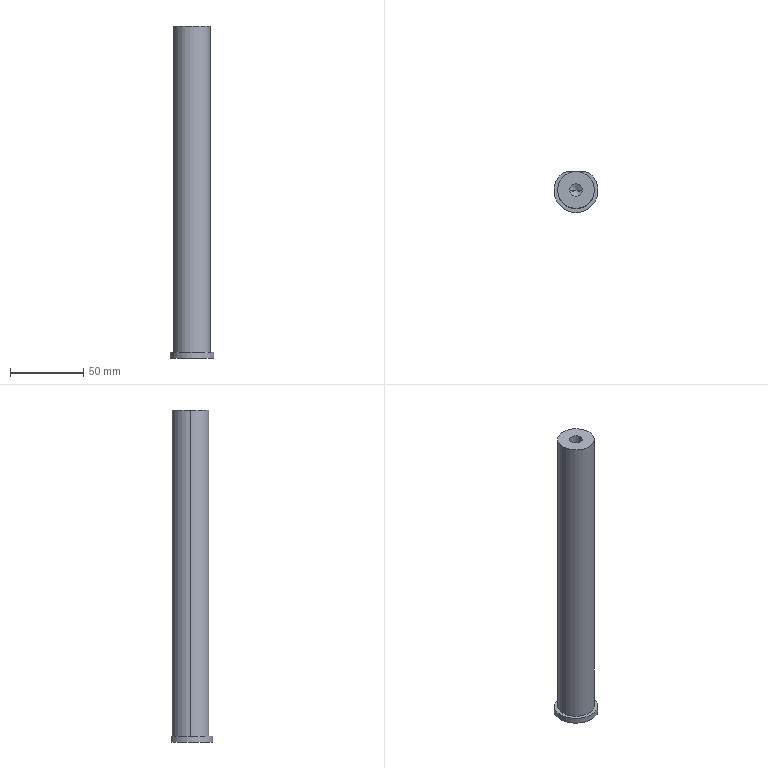Part | Creo | 1 solid | 13 faces | box 30 x 28 x 226 mm | volume 110529 mm3 | plane 6 | cylinder 5 | cone 2 | commonest cylinder face diameters 8.5 x2 25 x2 30 x1
STEP:
#1=CARTESIAN_POINT('',(0.,0.,0.));
#2=DIRECTION('',(0.,0.,1.));
#3=DIRECTION('',(1.,0.,0.));
#4=AXIS2_PLACEMENT_3D('',#1,#2,#3);
#5=CARTESIAN_POINT('',(108.255,195.804,-221.5));
#6=VERTEX_POINT('',#5);
#7=CARTESIAN_POINT('',(89.745,195.804,-221.5));
#8=VERTEX_POINT('',#7);
#9=CARTESIAN_POINT('',(99.,184.,-221.5));
#10=DIRECTION('',(0.,0.,-1.));
#11=DIRECTION('',(0.617,0.787,0.));
#12=AXIS2_PLACEMENT_3D('',#9,#10,#11);
#13=CIRCLE('',#12,15.);
#14=EDGE_CURVE('',#6,#8,#13,.T.);
#15=ORIENTED_EDGE('',*,*,#14,.F.);
#16=CARTESIAN_POINT('',(108.255,195.804,-225.5));
#17=VERTEX_POINT('',#16);
#18=CARTESIAN_POINT('',(108.255,195.804,-225.5));
#19=DIRECTION('',(0.,0.,1.));
#20=VECTOR('',#19,4.);
#21=LINE('',#18,#20);
#22=EDGE_CURVE('',#17,#6,#21,.T.);
#23=ORIENTED_EDGE('',*,*,#22,.F.);
#24=CARTESIAN_POINT('',(89.745,195.804,-225.5));
#25=VERTEX_POINT('',#24);
#26=CARTESIAN_POINT('',(99.,184.,-225.5));
#27=DIRECTION('',(0.,0.,1.));
#28=DIRECTION('',(-0.617,0.787,0.));
#29=AXIS2_PLACEMENT_3D('',#26,#27,#28);
#30=CIRCLE('',#29,15.);
#31=EDGE_CURVE('',#25,#17,#30,.T.);
#32=ORIENTED_EDGE('',*,*,#31,.F.);
#33=CARTESIAN_POINT('',(89.745,195.804,-221.5));
#34=DIRECTION('',(0.,0.,-1.));
#35=VECTOR('',#34,4.);
#36=LINE('',#33,#35);
#37=EDGE_CURVE('',#8,#25,#36,.T.);
#38=ORIENTED_EDGE('',*,*,#37,.F.);
#39=EDGE_LOOP('',(#15,#23,#32,#38));
#40=FACE_OUTER_BOUND('',#39,.F.);
#41=CARTESIAN_POINT('',(99.,184.,-221.5));
#42=DIRECTION('',(0.,0.,-1.));
#43=DIRECTION('',(1.,0.,0.));
#44=AXIS2_PLACEMENT_3D('',#41,#42,#43);
#45=CYLINDRICAL_SURFACE('',#44,15.);
#46=ADVANCED_FACE('',(#40),#45,.T.);
#47=CARTESIAN_POINT('',(104.792,197.,-221.5));
#48=VERTEX_POINT('',#47);
#49=CARTESIAN_POINT('',(93.208,197.,-221.5));
#50=VERTEX_POINT('',#49);
#51=CARTESIAN_POINT('',(104.792,197.,-221.5));
#52=DIRECTION('',(-1.,0.,0.));
#53=VECTOR('',#52,11.584);
#54=LINE('',#51,#53);
#55=EDGE_CURVE('',#48,#50,#54,.T.);
#56=ORIENTED_EDGE('',*,*,#55,.F.);
#57=CARTESIAN_POINT('',(108.255,195.804,-221.5));
#58=DIRECTION('',(-0.9452,0.3264,0.));
#59=VECTOR('',#58,3.664);
#60=LINE('',#57,#59);
#61=EDGE_CURVE('',#6,#48,#60,.T.);
#62=ORIENTED_EDGE('',*,*,#61,.F.);
#63=ORIENTED_EDGE('',*,*,#14,.T.);
#64=CARTESIAN_POINT('',(93.208,197.,-221.5));
#65=DIRECTION('',(-0.9452,-0.3264,0.));
#66=VECTOR('',#65,3.664);
#67=LINE('',#64,#66);
#68=EDGE_CURVE('',#50,#8,#67,.T.);
#69=ORIENTED_EDGE('',*,*,#68,.F.);
#70=EDGE_LOOP('',(#56,#62,#63,#69));
#71=FACE_OUTER_BOUND('',#70,.F.);
#72=CARTESIAN_POINT('',(111.5,184.,-221.5));
#73=VERTEX_POINT('',#72);
#74=CARTESIAN_POINT('',(86.5,184.,-221.5));
#75=VERTEX_POINT('',#74);
#76=CARTESIAN_POINT('',(99.,184.,-221.5));
#77=DIRECTION('',(0.,0.,-1.));
#78=DIRECTION('',(1.,0.,0.));
#79=AXIS2_PLACEMENT_3D('',#76,#77,#78);
#80=CIRCLE('',#79,12.5);
#81=EDGE_CURVE('',#73,#75,#80,.T.);
#82=ORIENTED_EDGE('',*,*,#81,.F.);
#83=CARTESIAN_POINT('',(99.,184.,-221.5));
#84=DIRECTION('',(0.,0.,-1.));
#85=DIRECTION('',(-1.,0.,0.));
#86=AXIS2_PLACEMENT_3D('',#83,#84,#85);
#87=CIRCLE('',#86,12.5);
#88=EDGE_CURVE('',#75,#73,#87,.T.);
#89=ORIENTED_EDGE('',*,*,#88,.F.);
#90=EDGE_LOOP('',(#82,#89));
#91=FACE_BOUND('',#90,.F.);
#92=CARTESIAN_POINT('',(99.,184.,-221.5));
#93=DIRECTION('',(0.,0.,1.));
#94=DIRECTION('',(-1.,0.,0.));
#95=AXIS2_PLACEMENT_3D('',#92,#93,#94);
#96=PLANE('',#95);
#97=ADVANCED_FACE('',(#71,#91),#96,.T.);
#98=CARTESIAN_POINT('',(86.5,184.,0.5));
#99=VERTEX_POINT('',#98);
#100=CARTESIAN_POINT('',(111.5,184.,0.5));
#101=VERTEX_POINT('',#100);
#102=CARTESIAN_POINT('',(99.,184.,0.5));
#103=DIRECTION('',(0.,0.,1.));
#104=DIRECTION('',(-1.,0.,0.));
#105=AXIS2_PLACEMENT_3D('',#102,#103,#104);
#106=CIRCLE('',#105,12.5);
#107=EDGE_CURVE('',#99,#101,#106,.T.);
#108=ORIENTED_EDGE('',*,*,#107,.T.);
#109=CARTESIAN_POINT('',(111.5,184.,-221.5));
#110=DIRECTION('',(0.,0.,1.));
#111=VECTOR('',#110,222.);
#112=LINE('',#109,#111);
#113=EDGE_CURVE('',#73,#101,#112,.T.);
#114=ORIENTED_EDGE('',*,*,#113,.F.);
#115=ORIENTED_EDGE('',*,*,#81,.T.);
#116=CARTESIAN_POINT('',(86.5,184.,-221.5));
#117=DIRECTION('',(0.,0.,1.));
#118=VECTOR('',#117,222.);
#119=LINE('',#116,#118);
#120=EDGE_CURVE('',#75,#99,#119,.T.);
#121=ORIENTED_EDGE('',*,*,#120,.T.);
#122=EDGE_LOOP('',(#108,#114,#115,#121));
#123=FACE_OUTER_BOUND('',#122,.F.);
#124=CARTESIAN_POINT('',(99.,184.,-221.5));
#125=DIRECTION('',(0.,0.,1.));
#126=DIRECTION('',(-1.,0.,0.));
#127=AXIS2_PLACEMENT_3D('',#124,#125,#126);
#128=CYLINDRICAL_SURFACE('',#127,12.5);
#129=ADVANCED_FACE('',(#123),#128,.T.);
#130=CARTESIAN_POINT('',(99.,184.,0.5));
#131=DIRECTION('',(0.,0.,1.));
#132=DIRECTION('',(1.,0.,0.));
#133=AXIS2_PLACEMENT_3D('',#130,#131,#132);
#134=CIRCLE('',#133,12.5);
#135=EDGE_CURVE('',#101,#99,#134,.T.);
#136=ORIENTED_EDGE('',*,*,#135,.F.);
#137=ORIENTED_EDGE('',*,*,#107,.F.);
#138=EDGE_LOOP('',(#136,#137));
#139=FACE_OUTER_BOUND('',#138,.F.);
#140=CARTESIAN_POINT('',(94.75,184.,0.5));
#141=VERTEX_POINT('',#140);
#142=CARTESIAN_POINT('',(103.25,184.,0.5));
#143=VERTEX_POINT('',#142);
#144=CARTESIAN_POINT('',(99.,184.,0.5));
#145=DIRECTION('',(0.,0.,-1.));
#146=DIRECTION('',(-1.,0.,0.));
#147=AXIS2_PLACEMENT_3D('',#144,#145,#146);
#148=CIRCLE('',#147,4.25);
#149=EDGE_CURVE('',#141,#143,#148,.T.);
#150=ORIENTED_EDGE('',*,*,#149,.F.);
#151=CARTESIAN_POINT('',(99.,184.,0.5));
#152=DIRECTION('',(0.,0.,-1.));
#153=DIRECTION('',(1.,0.,0.));
#154=AXIS2_PLACEMENT_3D('',#151,#152,#153);
#155=CIRCLE('',#154,4.25);
#156=EDGE_CURVE('',#143,#141,#155,.T.);
#157=ORIENTED_EDGE('',*,*,#156,.F.);
#158=EDGE_LOOP('',(#150,#157));
#159=FACE_BOUND('',#158,.F.);
#160=CARTESIAN_POINT('',(99.,184.,0.5));
#161=DIRECTION('',(0.,0.,1.));
#162=DIRECTION('',(-1.,0.,0.));
#163=AXIS2_PLACEMENT_3D('',#160,#161,#162);
#164=PLANE('',#163);
#165=ADVANCED_FACE('',(#139,#159),#164,.T.);
#166=CARTESIAN_POINT('',(103.25,184.,-19.5));
#167=VERTEX_POINT('',#166);
#168=CARTESIAN_POINT('',(94.75,184.,-19.5));
#169=VERTEX_POINT('',#168);
#170=CARTESIAN_POINT('',(99.,184.,-19.5));
#171=DIRECTION('',(0.,0.,1.));
#172=DIRECTION('',(1.,0.,0.));
#173=AXIS2_PLACEMENT_3D('',#170,#171,#172);
#174=CIRCLE('',#173,4.25);
#175=EDGE_CURVE('',#167,#169,#174,.T.);
#176=ORIENTED_EDGE('',*,*,#175,.T.);
#177=CARTESIAN_POINT('',(94.75,184.,0.5));
#178=DIRECTION('',(0.,0.,-1.));
#179=VECTOR('',#178,20.);
#180=LINE('',#177,#179);
#181=EDGE_CURVE('',#141,#169,#180,.T.);
#182=ORIENTED_EDGE('',*,*,#181,.F.);
#183=ORIENTED_EDGE('',*,*,#149,.T.);
#184=CARTESIAN_POINT('',(103.25,184.,0.5));
#185=DIRECTION('',(0.,0.,-1.));
#186=VECTOR('',#185,20.);
#187=LINE('',#184,#186);
#188=EDGE_CURVE('',#143,#167,#187,.T.);
#189=ORIENTED_EDGE('',*,*,#188,.T.);
#190=EDGE_LOOP('',(#176,#182,#183,#189));
#191=FACE_OUTER_BOUND('',#190,.F.);
#192=CARTESIAN_POINT('',(99.,184.,0.5));
#193=DIRECTION('',(0.,0.,-1.));
#194=DIRECTION('',(-1.,0.,0.));
#195=AXIS2_PLACEMENT_3D('',#192,#193,#194);
#196=CYLINDRICAL_SURFACE('',#195,4.25);
#197=ADVANCED_FACE('',(#191),#196,.F.);
#198=ORIENTED_EDGE('',*,*,#175,.F.);
#199=CARTESIAN_POINT('',(99.,184.,-22.054));
#200=VERTEX_POINT('',#199);
#201=CARTESIAN_POINT('',(99.,184.,-22.054));
#202=DIRECTION('',(0.8572,0.,0.515));
#203=VECTOR('',#202,4.958);
#204=LINE('',#201,#203);
#205=EDGE_CURVE('',#200,#167,#204,.T.);
#206=ORIENTED_EDGE('',*,*,#205,.F.);
#207=CARTESIAN_POINT('',(99.,184.,-22.054));
#208=DIRECTION('',(-0.8572,0.,0.515));
#209=VECTOR('',#208,4.958);
#210=LINE('',#207,#209);
#211=EDGE_CURVE('',#200,#169,#210,.T.);
#212=ORIENTED_EDGE('',*,*,#211,.T.);
#213=EDGE_LOOP('',(#198,#206,#212));
#214=FACE_OUTER_BOUND('',#213,.F.);
#215=CARTESIAN_POINT('',(99.,184.,-20.706));
#216=DIRECTION('',(0.,0.,1.));
#217=DIRECTION('',(1.,0.,0.));
#218=AXIS2_PLACEMENT_3D('',#215,#216,#217);
#219=CONICAL_SURFACE('',#218,2.243,59.);
#220=ADVANCED_FACE('',(#214),#219,.F.);
#221=CARTESIAN_POINT('',(99.,184.,-19.5));
#222=DIRECTION('',(0.,0.,1.));
#223=DIRECTION('',(-1.,0.,0.));
#224=AXIS2_PLACEMENT_3D('',#221,#222,#223);
#225=CIRCLE('',#224,4.25);
#226=EDGE_CURVE('',#169,#167,#225,.T.);
#227=ORIENTED_EDGE('',*,*,#226,.F.);
#228=ORIENTED_EDGE('',*,*,#211,.F.);
#229=ORIENTED_EDGE('',*,*,#205,.T.);
#230=EDGE_LOOP('',(#227,#228,#229));
#231=FACE_OUTER_BOUND('',#230,.F.);
#232=CARTESIAN_POINT('',(99.,184.,-20.706));
#233=DIRECTION('',(0.,0.,1.));
#234=DIRECTION('',(1.,0.,0.));
#235=AXIS2_PLACEMENT_3D('',#232,#233,#234);
#236=CONICAL_SURFACE('',#235,2.243,59.);
#237=ADVANCED_FACE('',(#231),#236,.F.);
#238=ORIENTED_EDGE('',*,*,#226,.T.);
#239=ORIENTED_EDGE('',*,*,#188,.F.);
#240=ORIENTED_EDGE('',*,*,#156,.T.);
#241=ORIENTED_EDGE('',*,*,#181,.T.);
#242=EDGE_LOOP('',(#238,#239,#240,#241));
#243=FACE_OUTER_BOUND('',#242,.F.);
#244=CARTESIAN_POINT('',(99.,184.,0.5));
#245=DIRECTION('',(0.,0.,-1.));
#246=DIRECTION('',(-1.,0.,0.));
#247=AXIS2_PLACEMENT_3D('',#244,#245,#246);
#248=CYLINDRICAL_SURFACE('',#247,4.25);
#249=ADVANCED_FACE('',(#243),#248,.F.);
#250=ORIENTED_EDGE('',*,*,#135,.T.);
#251=ORIENTED_EDGE('',*,*,#120,.F.);
#252=ORIENTED_EDGE('',*,*,#88,.T.);
#253=ORIENTED_EDGE('',*,*,#113,.T.);
#254=EDGE_LOOP('',(#250,#251,#252,#253));
#255=FACE_OUTER_BOUND('',#254,.F.);
#256=CARTESIAN_POINT('',(99.,184.,-221.5));
#257=DIRECTION('',(0.,0.,1.));
#258=DIRECTION('',(-1.,0.,0.));
#259=AXIS2_PLACEMENT_3D('',#256,#257,#258);
#260=CYLINDRICAL_SURFACE('',#259,12.5);
#261=ADVANCED_FACE('',(#255),#260,.T.);
#262=CARTESIAN_POINT('',(104.792,197.,-225.5));
#263=VERTEX_POINT('',#262);
#264=CARTESIAN_POINT('',(93.208,197.,-225.5));
#265=VERTEX_POINT('',#264);
#266=CARTESIAN_POINT('',(104.792,197.,-225.5));
#267=DIRECTION('',(-1.,0.,0.));
#268=VECTOR('',#267,11.584);
#269=LINE('',#266,#268);
#270=EDGE_CURVE('',#263,#265,#269,.T.);
#271=ORIENTED_EDGE('',*,*,#270,.F.);
#272=CARTESIAN_POINT('',(104.792,197.,-225.5));
#273=DIRECTION('',(0.,0.,1.));
#274=VECTOR('',#273,4.);
#275=LINE('',#272,#274);
#276=EDGE_CURVE('',#263,#48,#275,.T.);
#277=ORIENTED_EDGE('',*,*,#276,.T.);
#278=ORIENTED_EDGE('',*,*,#55,.T.);
#279=CARTESIAN_POINT('',(93.208,197.,-221.5));
#280=DIRECTION('',(0.,0.,-1.));
#281=VECTOR('',#280,4.);
#282=LINE('',#279,#281);
#283=EDGE_CURVE('',#50,#265,#282,.T.);
#284=ORIENTED_EDGE('',*,*,#283,.T.);
#285=EDGE_LOOP('',(#271,#277,#278,#284));
#286=FACE_OUTER_BOUND('',#285,.F.);
#287=CARTESIAN_POINT('',(99.,197.,-225.5));
#288=DIRECTION('',(0.,1.,0.));
#289=DIRECTION('',(0.,0.,1.));
#290=AXIS2_PLACEMENT_3D('',#287,#288,#289);
#291=PLANE('',#290);
#292=ADVANCED_FACE('',(#286),#291,.T.);
#293=ORIENTED_EDGE('',*,*,#31,.T.);
#294=CARTESIAN_POINT('',(104.792,197.,-225.5));
#295=DIRECTION('',(0.9452,-0.3264,0.));
#296=VECTOR('',#295,3.664);
#297=LINE('',#294,#296);
#298=EDGE_CURVE('',#263,#17,#297,.T.);
#299=ORIENTED_EDGE('',*,*,#298,.F.);
#300=ORIENTED_EDGE('',*,*,#270,.T.);
#301=CARTESIAN_POINT('',(89.745,195.804,-225.5));
#302=DIRECTION('',(0.9452,0.3264,0.));
#303=VECTOR('',#302,3.664);
#304=LINE('',#301,#303);
#305=EDGE_CURVE('',#25,#265,#304,.T.);
#306=ORIENTED_EDGE('',*,*,#305,.F.);
#307=EDGE_LOOP('',(#293,#299,#300,#306));
#308=FACE_OUTER_BOUND('',#307,.F.);
#309=CARTESIAN_POINT('',(99.,184.,-225.5));
#310=DIRECTION('',(0.,0.,1.));
#311=DIRECTION('',(-1.,0.,0.));
#312=AXIS2_PLACEMENT_3D('',#309,#310,#311);
#313=PLANE('',#312);
#314=ADVANCED_FACE('',(#308),#313,.F.);
#315=ORIENTED_EDGE('',*,*,#298,.T.);
#316=ORIENTED_EDGE('',*,*,#22,.T.);
#317=ORIENTED_EDGE('',*,*,#61,.T.);
#318=ORIENTED_EDGE('',*,*,#276,.F.);
#319=EDGE_LOOP('',(#315,#316,#317,#318));
#320=FACE_OUTER_BOUND('',#319,.F.);
#321=CARTESIAN_POINT('',(108.255,195.804,-221.5));
#322=DIRECTION('',(0.3264,0.9452,0.));
#323=DIRECTION('',(0.,0.,-1.));
#324=AXIS2_PLACEMENT_3D('',#321,#322,#323);
#325=PLANE('',#324);
#326=ADVANCED_FACE('',(#320),#325,.T.);
#327=ORIENTED_EDGE('',*,*,#68,.T.);
#328=ORIENTED_EDGE('',*,*,#37,.T.);
#329=ORIENTED_EDGE('',*,*,#305,.T.);
#330=ORIENTED_EDGE('',*,*,#283,.F.);
#331=EDGE_LOOP('',(#327,#328,#329,#330));
#332=FACE_OUTER_BOUND('',#331,.F.);
#333=CARTESIAN_POINT('',(89.745,195.804,-221.5));
#334=DIRECTION('',(0.3264,-0.9452,0.));
#335=DIRECTION('',(0.,0.,-1.));
#336=AXIS2_PLACEMENT_3D('',#333,#334,#335);
#337=PLANE('',#336);
#338=ADVANCED_FACE('',(#332),#337,.F.);
#339=CLOSED_SHELL('',(#46,#97,#129,#165,#197,#220,#237,#249,#261,#292,#314,#326,#338));
#340=MANIFOLD_SOLID_BREP('',#339);
#341=(LENGTH_UNIT()NAMED_UNIT(*)SI_UNIT(.MILLI.,.METRE.));
#342=UNCERTAINTY_MEASURE_WITH_UNIT(LENGTH_MEASURE(0.02297),#341,'','');
#343=(NAMED_UNIT(*)PLANE_ANGLE_UNIT()SI_UNIT($,.RADIAN.));
#344=PLANE_ANGLE_MEASURE_WITH_UNIT(PLANE_ANGLE_MEASURE(0.01745),#343);
#345=(CONVERSION_BASED_UNIT('DEGREE',#344)NAMED_UNIT(*)PLANE_ANGLE_UNIT());
#346=(NAMED_UNIT(*)SI_UNIT($,.STERADIAN.)SOLID_ANGLE_UNIT());
#347=(GEOMETRIC_REPRESENTATION_CONTEXT(3)GLOBAL_UNCERTAINTY_ASSIGNED_CONTEXT((#342))GLOBAL_UNIT_ASSIGNED_CONTEXT((#341,#345,#346))REPRESENTATION_CONTEXT('',''));
#348=ADVANCED_BREP_SHAPE_REPRESENTATION('',(#4,#340),#347);